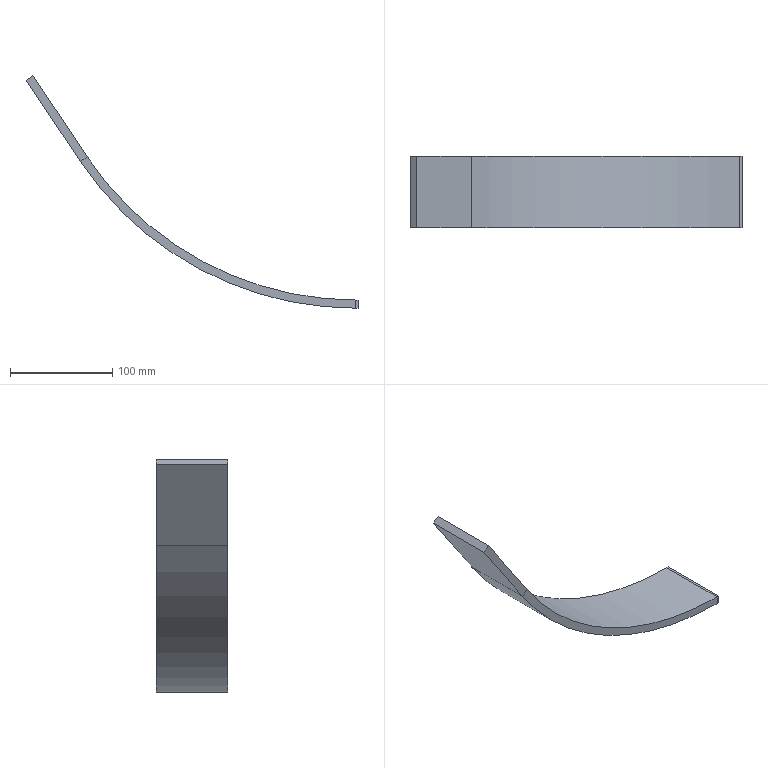Part | SolidWorks | features FlatPattern 1, SM3dBend 1, SMBaseFlange 1, SheetMetal 1 | 1 solid | 14 faces | box 325.308 x 70 x 227.668 mm | volume 230832 mm3 | plane 12 | cylinder 2 | commonest cylinder face diameters 634 x1 650 x1
STEP:
#1=CARTESIAN_POINT('',(146.936,70.,140.195));
#2=VERTEX_POINT('',#1);
#3=CARTESIAN_POINT('',(93.533,70.,219.668));
#4=VERTEX_POINT('',#3);
#5=CARTESIAN_POINT('',(93.533,70.,219.668));
#6=DIRECTION('',(-0.5577,0.,0.83));
#7=VECTOR('',#6,1000.);
#8=LINE('',#5,#7);
#9=EDGE_CURVE('',#2,#4,#8,.T.);
#10=ORIENTED_EDGE('',*,*,#9,.F.);
#11=CARTESIAN_POINT('',(140.296,70.,135.733));
#12=VERTEX_POINT('',#11);
#13=CARTESIAN_POINT('',(140.296,70.,135.733));
#14=DIRECTION('',(-0.83,0.,-0.5577));
#15=VECTOR('',#14,1000.);
#16=LINE('',#13,#15);
#17=EDGE_CURVE('',#2,#12,#16,.T.);
#18=ORIENTED_EDGE('',*,*,#17,.T.);
#19=CARTESIAN_POINT('',(86.892,70.,215.206));
#20=VERTEX_POINT('',#19);
#21=CARTESIAN_POINT('',(86.892,70.,215.206));
#22=DIRECTION('',(-0.5577,0.,0.83));
#23=VECTOR('',#22,1000.);
#24=LINE('',#21,#23);
#25=EDGE_CURVE('',#12,#20,#24,.T.);
#26=ORIENTED_EDGE('',*,*,#25,.T.);
#27=CARTESIAN_POINT('',(86.892,70.,215.206));
#28=DIRECTION('',(0.83,0.,0.5577));
#29=VECTOR('',#28,1000.);
#30=LINE('',#27,#29);
#31=EDGE_CURVE('',#20,#4,#30,.T.);
#32=ORIENTED_EDGE('',*,*,#31,.T.);
#33=EDGE_LOOP('',(#10,#18,#26,#32));
#34=FACE_OUTER_BOUND('',#33,.T.);
#35=CARTESIAN_POINT('',(86.892,70.,215.206));
#36=DIRECTION('',(0.,1.,0.));
#37=DIRECTION('',(0.83,0.,0.5577));
#38=AXIS2_PLACEMENT_3D('',#35,#36,#37);
#39=PLANE('',#38);
#40=ADVANCED_FACE('',(#34),#39,.T.);
#41=CARTESIAN_POINT('',(86.892,0.,215.206));
#42=VERTEX_POINT('',#41);
#43=CARTESIAN_POINT('',(140.296,0.,135.733));
#44=VERTEX_POINT('',#43);
#45=CARTESIAN_POINT('',(86.892,0.,215.206));
#46=DIRECTION('',(0.5577,0.,-0.83));
#47=VECTOR('',#46,1000.);
#48=LINE('',#45,#47);
#49=EDGE_CURVE('',#42,#44,#48,.T.);
#50=ORIENTED_EDGE('',*,*,#49,.T.);
#51=CARTESIAN_POINT('',(146.936,0.,140.195));
#52=VERTEX_POINT('',#51);
#53=CARTESIAN_POINT('',(140.296,0.,135.733));
#54=DIRECTION('',(0.83,0.,0.5577));
#55=VECTOR('',#54,1000.);
#56=LINE('',#53,#55);
#57=EDGE_CURVE('',#44,#52,#56,.T.);
#58=ORIENTED_EDGE('',*,*,#57,.T.);
#59=CARTESIAN_POINT('',(93.533,0.,219.668));
#60=VERTEX_POINT('',#59);
#61=CARTESIAN_POINT('',(93.533,0.,219.668));
#62=DIRECTION('',(0.5577,0.,-0.83));
#63=VECTOR('',#62,1000.);
#64=LINE('',#61,#63);
#65=EDGE_CURVE('',#60,#52,#64,.T.);
#66=ORIENTED_EDGE('',*,*,#65,.F.);
#67=CARTESIAN_POINT('',(86.892,0.,215.206));
#68=DIRECTION('',(0.83,0.,0.5577));
#69=VECTOR('',#68,1000.);
#70=LINE('',#67,#69);
#71=EDGE_CURVE('',#42,#60,#70,.T.);
#72=ORIENTED_EDGE('',*,*,#71,.F.);
#73=EDGE_LOOP('',(#50,#58,#66,#72));
#74=FACE_OUTER_BOUND('',#73,.T.);
#75=CARTESIAN_POINT('',(86.892,0.,215.206));
#76=DIRECTION('',(0.,-1.,0.));
#77=DIRECTION('',(-0.83,0.,-0.5577));
#78=AXIS2_PLACEMENT_3D('',#75,#76,#77);
#79=PLANE('',#78);
#80=ADVANCED_FACE('',(#74),#79,.T.);
#81=ORIENTED_EDGE('',*,*,#25,.F.);
#82=CARTESIAN_POINT('',(140.296,70.,135.733));
#83=DIRECTION('',(0.,-1.,0.));
#84=VECTOR('',#83,1000.);
#85=LINE('',#82,#84);
#86=EDGE_CURVE('',#12,#44,#85,.T.);
#87=ORIENTED_EDGE('',*,*,#86,.T.);
#88=ORIENTED_EDGE('',*,*,#49,.F.);
#89=CARTESIAN_POINT('',(86.892,0.,215.206));
#90=DIRECTION('',(0.,-1.,0.));
#91=VECTOR('',#90,1000.);
#92=LINE('',#89,#91);
#93=EDGE_CURVE('',#20,#42,#92,.T.);
#94=ORIENTED_EDGE('',*,*,#93,.F.);
#95=EDGE_LOOP('',(#81,#87,#88,#94));
#96=FACE_OUTER_BOUND('',#95,.T.);
#97=CARTESIAN_POINT('',(86.892,70.,215.206));
#98=DIRECTION('',(-0.83,0.,-0.5577));
#99=DIRECTION('',(-0.5577,0.,0.83));
#100=AXIS2_PLACEMENT_3D('',#97,#98,#99);
#101=PLANE('',#100);
#102=ADVANCED_FACE('',(#96),#101,.T.);
#103=CARTESIAN_POINT('',(93.533,0.,219.668));
#104=DIRECTION('',(0.,-1.,0.));
#105=VECTOR('',#104,1000.);
#106=LINE('',#103,#105);
#107=EDGE_CURVE('',#4,#60,#106,.T.);
#108=ORIENTED_EDGE('',*,*,#107,.F.);
#109=ORIENTED_EDGE('',*,*,#31,.F.);
#110=ORIENTED_EDGE('',*,*,#93,.T.);
#111=ORIENTED_EDGE('',*,*,#71,.T.);
#112=EDGE_LOOP('',(#108,#109,#110,#111));
#113=FACE_OUTER_BOUND('',#112,.T.);
#114=CARTESIAN_POINT('',(86.892,0.,215.206));
#115=DIRECTION('',(-0.5577,0.,0.83));
#116=DIRECTION('',(0.83,0.,0.5577));
#117=AXIS2_PLACEMENT_3D('',#114,#115,#116);
#118=PLANE('',#117);
#119=ADVANCED_FACE('',(#113),#118,.T.);
#120=CARTESIAN_POINT('',(146.936,70.,140.195));
#121=DIRECTION('',(0.,-1.,0.));
#122=VECTOR('',#121,1000.);
#123=LINE('',#120,#122);
#124=EDGE_CURVE('',#2,#52,#123,.T.);
#125=ORIENTED_EDGE('',*,*,#124,.F.);
#126=ORIENTED_EDGE('',*,*,#9,.T.);
#127=ORIENTED_EDGE('',*,*,#107,.T.);
#128=ORIENTED_EDGE('',*,*,#65,.T.);
#129=EDGE_LOOP('',(#125,#126,#127,#128));
#130=FACE_OUTER_BOUND('',#129,.T.);
#131=CARTESIAN_POINT('',(93.533,70.,219.668));
#132=DIRECTION('',(-0.83,0.,-0.5577));
#133=DIRECTION('',(-0.5577,0.,0.83));
#134=AXIS2_PLACEMENT_3D('',#131,#132,#133);
#135=PLANE('',#134);
#136=ADVANCED_FACE('',(#130),#135,.F.);
#137=CARTESIAN_POINT('',(412.2,0.,0.));
#138=VERTEX_POINT('',#137);
#139=CARTESIAN_POINT('',(412.2,70.,0.));
#140=VERTEX_POINT('',#139);
#141=CARTESIAN_POINT('',(412.2,0.,0.));
#142=DIRECTION('',(0.,1.,0.));
#143=VECTOR('',#142,1000.);
#144=LINE('',#141,#143);
#145=EDGE_CURVE('',#138,#140,#144,.T.);
#146=ORIENTED_EDGE('',*,*,#145,.F.);
#147=CARTESIAN_POINT('',(412.2,0.,-8.));
#148=VERTEX_POINT('',#147);
#149=CARTESIAN_POINT('',(412.2,0.,-8.));
#150=DIRECTION('',(0.,0.,1.));
#151=VECTOR('',#150,1000.);
#152=LINE('',#149,#151);
#153=EDGE_CURVE('',#148,#138,#152,.T.);
#154=ORIENTED_EDGE('',*,*,#153,.F.);
#155=CARTESIAN_POINT('',(412.2,70.,-8.));
#156=VERTEX_POINT('',#155);
#157=CARTESIAN_POINT('',(412.2,0.,-8.));
#158=DIRECTION('',(0.,1.,0.));
#159=VECTOR('',#158,1000.);
#160=LINE('',#157,#159);
#161=EDGE_CURVE('',#148,#156,#160,.T.);
#162=ORIENTED_EDGE('',*,*,#161,.T.);
#163=CARTESIAN_POINT('',(412.2,70.,-8.));
#164=DIRECTION('',(0.,0.,1.));
#165=VECTOR('',#164,1000.);
#166=LINE('',#163,#165);
#167=EDGE_CURVE('',#156,#140,#166,.T.);
#168=ORIENTED_EDGE('',*,*,#167,.T.);
#169=EDGE_LOOP('',(#146,#154,#162,#168));
#170=FACE_OUTER_BOUND('',#169,.T.);
#171=CARTESIAN_POINT('',(412.2,0.,-8.));
#172=DIRECTION('',(1.,0.,0.));
#173=DIRECTION('',(0.,0.,-1.));
#174=AXIS2_PLACEMENT_3D('',#171,#172,#173);
#175=PLANE('',#174);
#176=ADVANCED_FACE('',(#170),#175,.T.);
#177=CARTESIAN_POINT('',(410.05,70.,-8.));
#178=VERTEX_POINT('',#177);
#179=CARTESIAN_POINT('',(410.05,0.,-8.));
#180=VERTEX_POINT('',#179);
#181=CARTESIAN_POINT('',(410.05,70.,-8.));
#182=DIRECTION('',(0.,-1.,0.));
#183=VECTOR('',#182,1000.);
#184=LINE('',#181,#183);
#185=EDGE_CURVE('',#178,#180,#184,.T.);
#186=ORIENTED_EDGE('',*,*,#185,.F.);
#187=CARTESIAN_POINT('',(0.,70.,-8.));
#188=DIRECTION('',(-1.,0.,0.));
#189=VECTOR('',#188,1000.);
#190=LINE('',#187,#189);
#191=EDGE_CURVE('',#156,#178,#190,.T.);
#192=ORIENTED_EDGE('',*,*,#191,.F.);
#193=ORIENTED_EDGE('',*,*,#161,.F.);
#194=CARTESIAN_POINT('',(0.,0.,-8.));
#195=DIRECTION('',(1.,0.,0.));
#196=VECTOR('',#195,1000.);
#197=LINE('',#194,#196);
#198=EDGE_CURVE('',#180,#148,#197,.T.);
#199=ORIENTED_EDGE('',*,*,#198,.F.);
#200=EDGE_LOOP('',(#186,#192,#193,#199));
#201=FACE_OUTER_BOUND('',#200,.T.);
#202=CARTESIAN_POINT('',(0.,70.,-8.));
#203=DIRECTION('',(0.,0.,-1.));
#204=DIRECTION('',(-1.,0.,0.));
#205=AXIS2_PLACEMENT_3D('',#202,#203,#204);
#206=PLANE('',#205);
#207=ADVANCED_FACE('',(#201),#206,.T.);
#208=CARTESIAN_POINT('',(410.05,70.,0.));
#209=VERTEX_POINT('',#208);
#210=CARTESIAN_POINT('',(410.05,70.,-8.));
#211=DIRECTION('',(0.,0.,-1.));
#212=VECTOR('',#211,1000.);
#213=LINE('',#210,#212);
#214=EDGE_CURVE('',#209,#178,#213,.T.);
#215=ORIENTED_EDGE('',*,*,#214,.F.);
#216=CARTESIAN_POINT('',(0.,70.,0.));
#217=DIRECTION('',(-1.,0.,0.));
#218=VECTOR('',#217,1000.);
#219=LINE('',#216,#218);
#220=EDGE_CURVE('',#140,#209,#219,.T.);
#221=ORIENTED_EDGE('',*,*,#220,.F.);
#222=ORIENTED_EDGE('',*,*,#167,.F.);
#223=ORIENTED_EDGE('',*,*,#191,.T.);
#224=EDGE_LOOP('',(#215,#221,#222,#223));
#225=FACE_OUTER_BOUND('',#224,.T.);
#226=CARTESIAN_POINT('',(0.,70.,-8.));
#227=DIRECTION('',(0.,1.,0.));
#228=DIRECTION('',(0.,0.,1.));
#229=AXIS2_PLACEMENT_3D('',#226,#227,#228);
#230=PLANE('',#229);
#231=ADVANCED_FACE('',(#225),#230,.T.);
#232=ORIENTED_EDGE('',*,*,#220,.T.);
#233=CARTESIAN_POINT('',(410.05,0.,0.));
#234=VERTEX_POINT('',#233);
#235=CARTESIAN_POINT('',(410.05,70.,0.));
#236=DIRECTION('',(0.,-1.,0.));
#237=VECTOR('',#236,1000.);
#238=LINE('',#235,#237);
#239=EDGE_CURVE('',#209,#234,#238,.T.);
#240=ORIENTED_EDGE('',*,*,#239,.T.);
#241=CARTESIAN_POINT('',(0.,0.,0.));
#242=DIRECTION('',(1.,0.,0.));
#243=VECTOR('',#242,1000.);
#244=LINE('',#241,#243);
#245=EDGE_CURVE('',#234,#138,#244,.T.);
#246=ORIENTED_EDGE('',*,*,#245,.T.);
#247=ORIENTED_EDGE('',*,*,#145,.T.);
#248=EDGE_LOOP('',(#232,#240,#246,#247));
#249=FACE_OUTER_BOUND('',#248,.T.);
#250=CARTESIAN_POINT('',(0.,70.,0.));
#251=DIRECTION('',(0.,0.,-1.));
#252=DIRECTION('',(-1.,0.,0.));
#253=AXIS2_PLACEMENT_3D('',#250,#251,#252);
#254=PLANE('',#253);
#255=ADVANCED_FACE('',(#249),#254,.F.);
#256=CARTESIAN_POINT('',(410.05,0.,-8.));
#257=DIRECTION('',(0.,0.,1.));
#258=VECTOR('',#257,1000.);
#259=LINE('',#256,#258);
#260=EDGE_CURVE('',#180,#234,#259,.T.);
#261=ORIENTED_EDGE('',*,*,#260,.F.);
#262=ORIENTED_EDGE('',*,*,#198,.T.);
#263=ORIENTED_EDGE('',*,*,#153,.T.);
#264=ORIENTED_EDGE('',*,*,#245,.F.);
#265=EDGE_LOOP('',(#261,#262,#263,#264));
#266=FACE_OUTER_BOUND('',#265,.T.);
#267=CARTESIAN_POINT('',(0.,0.,-8.));
#268=DIRECTION('',(0.,-1.,0.));
#269=DIRECTION('',(0.,0.,-1.));
#270=AXIS2_PLACEMENT_3D('',#267,#268,#269);
#271=PLANE('',#270);
#272=ADVANCED_FACE('',(#266),#271,.T.);
#273=ORIENTED_EDGE('',*,*,#17,.F.);
#274=CARTESIAN_POINT('',(410.05,70.,317.));
#275=DIRECTION('',(0.,-1.,0.));
#276=DIRECTION('',(0.,0.,1.));
#277=AXIS2_PLACEMENT_3D('',#274,#275,#276);
#278=CIRCLE('',#277,317.);
#279=EDGE_CURVE('',#2,#209,#278,.T.);
#280=ORIENTED_EDGE('',*,*,#279,.T.);
#281=ORIENTED_EDGE('',*,*,#214,.T.);
#282=CARTESIAN_POINT('',(410.05,70.,317.));
#283=DIRECTION('',(0.,-1.,0.));
#284=DIRECTION('',(0.,0.,1.));
#285=AXIS2_PLACEMENT_3D('',#282,#283,#284);
#286=CIRCLE('',#285,325.);
#287=EDGE_CURVE('',#12,#178,#286,.T.);
#288=ORIENTED_EDGE('',*,*,#287,.F.);
#289=EDGE_LOOP('',(#273,#280,#281,#288));
#290=FACE_OUTER_BOUND('',#289,.T.);
#291=CARTESIAN_POINT('',(410.05,70.,317.));
#292=DIRECTION('',(0.,1.,0.));
#293=DIRECTION('',(0.,0.,1.));
#294=AXIS2_PLACEMENT_3D('',#291,#292,#293);
#295=PLANE('',#294);
#296=ADVANCED_FACE('',(#290),#295,.T.);
#297=ORIENTED_EDGE('',*,*,#185,.T.);
#298=CARTESIAN_POINT('',(410.05,0.,317.));
#299=DIRECTION('',(0.,1.,0.));
#300=DIRECTION('',(0.,0.,-1.));
#301=AXIS2_PLACEMENT_3D('',#298,#299,#300);
#302=CIRCLE('',#301,325.);
#303=EDGE_CURVE('',#180,#44,#302,.T.);
#304=ORIENTED_EDGE('',*,*,#303,.T.);
#305=ORIENTED_EDGE('',*,*,#86,.F.);
#306=ORIENTED_EDGE('',*,*,#287,.T.);
#307=EDGE_LOOP('',(#297,#304,#305,#306));
#308=FACE_OUTER_BOUND('',#307,.T.);
#309=CARTESIAN_POINT('',(410.05,-287.101,317.));
#310=DIRECTION('',(0.,1.,0.));
#311=DIRECTION('',(0.,0.,1.));
#312=AXIS2_PLACEMENT_3D('',#309,#310,#311);
#313=CYLINDRICAL_SURFACE('',#312,325.);
#314=ADVANCED_FACE('',(#308),#313,.T.);
#315=CARTESIAN_POINT('',(410.05,0.,317.));
#316=DIRECTION('',(0.,1.,0.));
#317=DIRECTION('',(0.,0.,1.));
#318=AXIS2_PLACEMENT_3D('',#315,#316,#317);
#319=CIRCLE('',#318,317.);
#320=EDGE_CURVE('',#234,#52,#319,.T.);
#321=ORIENTED_EDGE('',*,*,#320,.T.);
#322=ORIENTED_EDGE('',*,*,#57,.F.);
#323=ORIENTED_EDGE('',*,*,#303,.F.);
#324=ORIENTED_EDGE('',*,*,#260,.T.);
#325=EDGE_LOOP('',(#321,#322,#323,#324));
#326=FACE_OUTER_BOUND('',#325,.T.);
#327=CARTESIAN_POINT('',(410.05,0.,317.));
#328=DIRECTION('',(0.,-1.,0.));
#329=DIRECTION('',(0.,0.,-1.));
#330=AXIS2_PLACEMENT_3D('',#327,#328,#329);
#331=PLANE('',#330);
#332=ADVANCED_FACE('',(#326),#331,.T.);
#333=ORIENTED_EDGE('',*,*,#239,.F.);
#334=ORIENTED_EDGE('',*,*,#279,.F.);
#335=ORIENTED_EDGE('',*,*,#124,.T.);
#336=ORIENTED_EDGE('',*,*,#320,.F.);
#337=EDGE_LOOP('',(#333,#334,#335,#336));
#338=FACE_OUTER_BOUND('',#337,.T.);
#339=CARTESIAN_POINT('',(410.05,-287.101,317.));
#340=DIRECTION('',(0.,1.,0.));
#341=DIRECTION('',(0.,0.,1.));
#342=AXIS2_PLACEMENT_3D('',#339,#340,#341);
#343=CYLINDRICAL_SURFACE('',#342,317.);
#344=ADVANCED_FACE('',(#338),#343,.F.);
#345=CLOSED_SHELL('',(#40,#80,#102,#119,#136,#176,#207,#231,#255,#272,#296,#314,#332,#344));
#346=MANIFOLD_SOLID_BREP('',#345);
#347=CARTESIAN_POINT('',(0.,0.,0.));
#348=DIRECTION('',(0.,0.,1.));
#349=DIRECTION('',(1.,0.,0.));
#350=AXIS2_PLACEMENT_3D('',#347,#348,#349);
#351=(LENGTH_UNIT()NAMED_UNIT(*)SI_UNIT(.MILLI.,.METRE.));
#352=UNCERTAINTY_MEASURE_WITH_UNIT(LENGTH_MEASURE(0.00001),#351,'','');
#353=(NAMED_UNIT(*)PLANE_ANGLE_UNIT()SI_UNIT($,.RADIAN.));
#354=(NAMED_UNIT(*)SI_UNIT($,.STERADIAN.)SOLID_ANGLE_UNIT());
#355=(GEOMETRIC_REPRESENTATION_CONTEXT(3)GLOBAL_UNCERTAINTY_ASSIGNED_CONTEXT((#352))GLOBAL_UNIT_ASSIGNED_CONTEXT((#351,#353,#354))REPRESENTATION_CONTEXT('',''));
#356=ADVANCED_BREP_SHAPE_REPRESENTATION('',(#346,#350),#355);